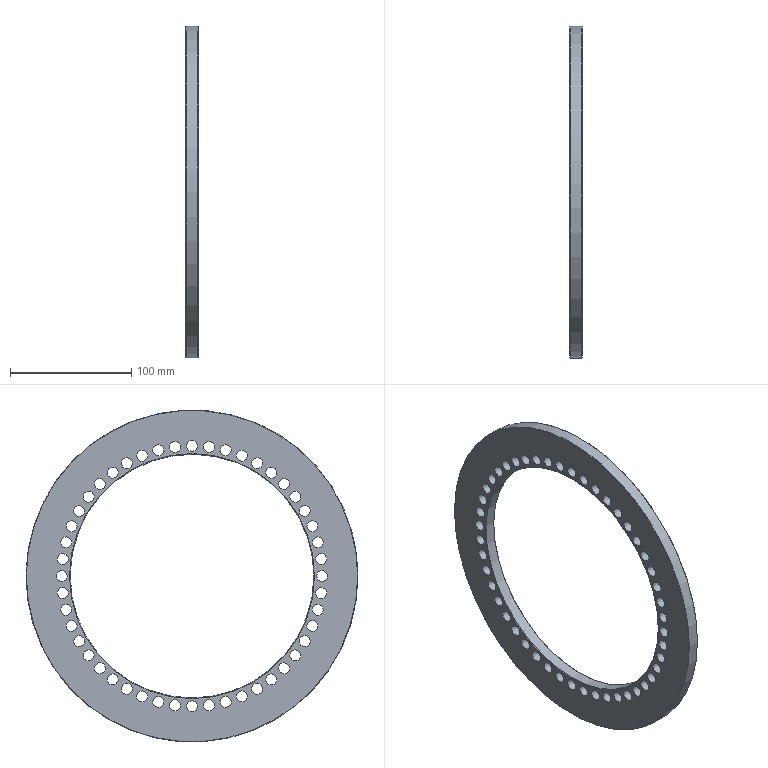Part | STEP file | Part [2] | 1 solid | 56 faces | box 10.03 x 274 x 274 mm | volume 241970 mm3 | cylinder 50 | cone 4 | plane 2 | commonest cylinder face diameters 9 x48 201.1 x1 274 x1